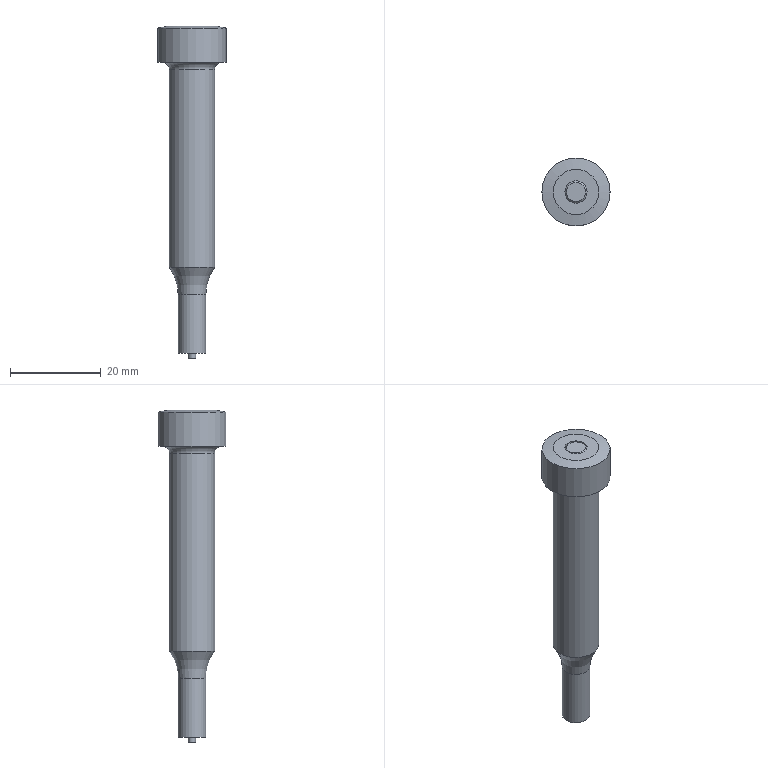Part | NX | features APJAS10-90-P6.08_2 2 | 1 solid | 20 faces | box 15 x 15 x 73 mm | volume 5513 mm3 | cylinder 8 | plane 7 | torus 2 | cone 2 | spline 1 | commonest cylinder face diameters 1.6 x1 1.8 x1 4.2 x1 4.4 x1 4.9 x1 6.08 x1
STEP:
#1=CARTESIAN_POINT('',(660.878,-22.569,60.5));
#2=VERTEX_POINT('',#1);
#3=CARTESIAN_POINT('',(665.878,-22.569,60.5));
#4=DIRECTION('',(0.,0.,1.));
#5=DIRECTION('',(1.,0.,0.));
#6=AXIS2_PLACEMENT_3D('',#3,#4,#5);
#7=CIRCLE('',#6,5.);
#8=EDGE_CURVE('',#2,#2,#7,.T.);
#9=ORIENTED_EDGE('',*,*,#8,.F.);
#10=EDGE_LOOP('',(#9));
#11=FACE_BOUND('',#10,.T.);
#12=CARTESIAN_POINT('',(670.878,-22.569,16.946));
#13=VERTEX_POINT('',#12);
#14=CARTESIAN_POINT('',(665.878,-22.569,16.946));
#15=DIRECTION('',(0.,0.,1.));
#16=DIRECTION('',(-1.,0.,0.));
#17=AXIS2_PLACEMENT_3D('',#14,#15,#16);
#18=CIRCLE('',#17,5.);
#19=EDGE_CURVE('',#13,#13,#18,.T.);
#20=ORIENTED_EDGE('',*,*,#19,.T.);
#21=EDGE_LOOP('',(#20));
#22=FACE_BOUND('',#21,.T.);
#23=CARTESIAN_POINT('',(665.878,-22.569,45.5));
#24=DIRECTION('',(0.,0.,-1.));
#25=DIRECTION('',(1.,0.,0.));
#26=AXIS2_PLACEMENT_3D('',#23,#24,#25);
#27=CYLINDRICAL_SURFACE('',#26,5.);
#28=ADVANCED_FACE('',(#11,#22),#27,.T.);
#29=CARTESIAN_POINT('',(664.978,-22.569,26.));
#30=VERTEX_POINT('',#29);
#31=CARTESIAN_POINT('',(665.878,-22.569,26.));
#32=DIRECTION('',(0.,0.,1.));
#33=DIRECTION('',(-1.,0.,0.));
#34=AXIS2_PLACEMENT_3D('',#31,#32,#33);
#35=CIRCLE('',#34,0.9);
#36=EDGE_CURVE('',#30,#30,#35,.T.);
#37=ORIENTED_EDGE('',*,*,#36,.T.);
#38=EDGE_LOOP('',(#37));
#39=FACE_BOUND('',#38,.T.);
#40=CARTESIAN_POINT('',(664.978,-22.569,-2.));
#41=VERTEX_POINT('',#40);
#42=CARTESIAN_POINT('',(665.878,-22.569,-2.));
#43=DIRECTION('',(0.,0.,1.));
#44=DIRECTION('',(-1.,0.,0.));
#45=AXIS2_PLACEMENT_3D('',#42,#43,#44);
#46=CIRCLE('',#45,0.9);
#47=EDGE_CURVE('',#41,#41,#46,.T.);
#48=ORIENTED_EDGE('',*,*,#47,.F.);
#49=EDGE_LOOP('',(#48));
#50=FACE_BOUND('',#49,.T.);
#51=CARTESIAN_POINT('',(665.878,-22.569,12.));
#52=DIRECTION('',(0.,0.,-1.));
#53=DIRECTION('',(1.,0.,0.));
#54=AXIS2_PLACEMENT_3D('',#51,#52,#53);
#55=CYLINDRICAL_SURFACE('',#54,0.9);
#56=ADVANCED_FACE('',(#39,#50),#55,.F.);
#57=CARTESIAN_POINT('',(668.328,-22.569,69.632));
#58=VERTEX_POINT('',#57);
#59=CARTESIAN_POINT('',(665.878,-22.569,69.632));
#60=DIRECTION('',(0.,0.,1.));
#61=DIRECTION('',(1.,0.,0.));
#62=AXIS2_PLACEMENT_3D('',#59,#60,#61);
#63=CIRCLE('',#62,2.45);
#64=EDGE_CURVE('',#58,#58,#63,.T.);
#65=ORIENTED_EDGE('',*,*,#64,.F.);
#66=EDGE_LOOP('',(#65));
#67=FACE_BOUND('',#66,.T.);
#68=CARTESIAN_POINT('',(663.428,-22.569,70.));
#69=VERTEX_POINT('',#68);
#70=CARTESIAN_POINT('',(665.878,-22.569,70.));
#71=DIRECTION('',(0.,0.,-1.));
#72=DIRECTION('',(-1.,0.,0.));
#73=AXIS2_PLACEMENT_3D('',#70,#71,#72);
#74=CIRCLE('',#73,2.45);
#75=EDGE_CURVE('',#69,#69,#74,.T.);
#76=ORIENTED_EDGE('',*,*,#75,.F.);
#77=EDGE_LOOP('',(#76));
#78=FACE_BOUND('',#77,.T.);
#79=CARTESIAN_POINT('',(665.878,-22.569,68.775));
#80=DIRECTION('',(0.,0.,-1.));
#81=DIRECTION('',(1.,0.,0.));
#82=AXIS2_PLACEMENT_3D('',#79,#80,#81);
#83=CYLINDRICAL_SURFACE('',#82,2.45);
#84=ADVANCED_FACE('',(#67,#78),#83,.F.);
#85=ORIENTED_EDGE('',*,*,#8,.T.);
#86=EDGE_LOOP('',(#85));
#87=FACE_BOUND('',#86,.T.);
#88=CARTESIAN_POINT('',(659.378,-22.569,62.));
#89=VERTEX_POINT('',#88);
#90=CARTESIAN_POINT('',(665.878,-22.569,62.));
#91=DIRECTION('',(0.,0.,-1.));
#92=DIRECTION('',(1.,0.,0.));
#93=AXIS2_PLACEMENT_3D('',#90,#91,#92);
#94=CIRCLE('',#93,6.5);
#95=EDGE_CURVE('',#89,#89,#94,.T.);
#96=ORIENTED_EDGE('',*,*,#95,.T.);
#97=EDGE_LOOP('',(#96));
#98=FACE_BOUND('',#97,.T.);
#99=CARTESIAN_POINT('',(665.878,-22.569,60.5));
#100=DIRECTION('',(0.,0.,1.));
#101=DIRECTION('',(-1.,0.,0.));
#102=AXIS2_PLACEMENT_3D('',#99,#100,#101);
#103=TOROIDAL_SURFACE('',#102,6.5,1.5);
#104=ADVANCED_FACE('',(#87,#98),#103,.F.);
#105=CARTESIAN_POINT('',(658.378,-22.569,62.));
#106=VERTEX_POINT('',#105);
#107=CARTESIAN_POINT('',(665.878,-22.569,62.));
#108=DIRECTION('',(0.,0.,-1.));
#109=DIRECTION('',(-1.,0.,0.));
#110=AXIS2_PLACEMENT_3D('',#107,#108,#109);
#111=CIRCLE('',#110,7.5);
#112=EDGE_CURVE('',#106,#106,#111,.T.);
#113=ORIENTED_EDGE('',*,*,#112,.T.);
#114=EDGE_LOOP('',(#113));
#115=FACE_BOUND('',#114,.T.);
#116=ORIENTED_EDGE('',*,*,#95,.F.);
#117=EDGE_LOOP('',(#116));
#118=FACE_BOUND('',#117,.T.);
#119=CARTESIAN_POINT('',(665.878,-22.569,62.));
#120=DIRECTION('',(0.,0.,-1.));
#121=DIRECTION('',(1.,0.,0.));
#122=AXIS2_PLACEMENT_3D('',#119,#120,#121);
#123=PLANE('',#122);
#124=ADVANCED_FACE('',(#115,#118),#123,.T.);
#125=CARTESIAN_POINT('',(662.838,-22.569,11.));
#126=VERTEX_POINT('',#125);
#127=CARTESIAN_POINT('',(665.878,-22.569,11.));
#128=DIRECTION('',(0.,0.,1.));
#129=DIRECTION('',(-1.,0.,0.));
#130=AXIS2_PLACEMENT_3D('',#127,#128,#129);
#131=CIRCLE('',#130,3.04);
#132=EDGE_CURVE('',#126,#126,#131,.T.);
#133=ORIENTED_EDGE('',*,*,#132,.T.);
#134=EDGE_LOOP('',(#133));
#135=FACE_BOUND('',#134,.T.);
#136=ORIENTED_EDGE('',*,*,#19,.F.);
#137=EDGE_LOOP('',(#136));
#138=FACE_BOUND('',#137,.T.);
#139=CARTESIAN_POINT('',(665.878,-22.569,11.));
#140=DIRECTION('',(0.,0.,-1.));
#141=DIRECTION('',(1.,0.,0.));
#142=AXIS2_PLACEMENT_3D('',#139,#140,#141);
#143=TOROIDAL_SURFACE('',#142,13.04,10.);
#144=ADVANCED_FACE('',(#135,#138),#143,.F.);
#145=CARTESIAN_POINT('',(658.378,-22.569,69.559));
#146=VERTEX_POINT('',#145);
#147=CARTESIAN_POINT('',(665.878,-22.569,69.559));
#148=DIRECTION('',(0.,0.,1.));
#149=DIRECTION('',(1.,0.,0.));
#150=AXIS2_PLACEMENT_3D('',#147,#148,#149);
#151=CIRCLE('',#150,7.5);
#152=EDGE_CURVE('',#146,#146,#151,.T.);
#153=ORIENTED_EDGE('',*,*,#152,.T.);
#154=EDGE_LOOP('',(#153));
#155=FACE_BOUND('',#154,.T.);
#156=CARTESIAN_POINT('',(660.878,-22.569,70.));
#157=VERTEX_POINT('',#156);
#158=CARTESIAN_POINT('',(665.878,-22.569,70.));
#159=DIRECTION('',(0.,0.,-1.));
#160=DIRECTION('',(1.,0.,0.));
#161=AXIS2_PLACEMENT_3D('',#158,#159,#160);
#162=CIRCLE('',#161,5.);
#163=EDGE_CURVE('',#157,#157,#162,.T.);
#164=ORIENTED_EDGE('',*,*,#163,.T.);
#165=EDGE_LOOP('',(#164));
#166=FACE_BOUND('',#165,.T.);
#167=CARTESIAN_POINT('',(665.878,-22.569,70.));
#168=DIRECTION('',(0.,0.,-1.));
#169=DIRECTION('',(-1.,0.,0.));
#170=AXIS2_PLACEMENT_3D('',#167,#168,#169);
#171=CONICAL_SURFACE('',#170,5.,1.396);
#172=ADVANCED_FACE('',(#155,#166),#171,.T.);
#173=ORIENTED_EDGE('',*,*,#112,.F.);
#174=EDGE_LOOP('',(#173));
#175=FACE_BOUND('',#174,.T.);
#176=ORIENTED_EDGE('',*,*,#152,.F.);
#177=EDGE_LOOP('',(#176));
#178=FACE_BOUND('',#177,.T.);
#179=CARTESIAN_POINT('',(665.878,-22.569,66.));
#180=DIRECTION('',(0.,0.,-1.));
#181=DIRECTION('',(1.,0.,0.));
#182=AXIS2_PLACEMENT_3D('',#179,#180,#181);
#183=CYLINDRICAL_SURFACE('',#182,7.5);
#184=ADVANCED_FACE('',(#175,#178),#183,.T.);
#185=ORIENTED_EDGE('',*,*,#75,.T.);
#186=EDGE_LOOP('',(#185));
#187=FACE_BOUND('',#186,.T.);
#188=ORIENTED_EDGE('',*,*,#163,.F.);
#189=EDGE_LOOP('',(#188));
#190=FACE_BOUND('',#189,.T.);
#191=CARTESIAN_POINT('',(665.878,-22.569,70.));
#192=DIRECTION('',(0.,0.,1.));
#193=DIRECTION('',(-1.,0.,0.));
#194=AXIS2_PLACEMENT_3D('',#191,#192,#193);
#195=PLANE('',#194);
#196=ADVANCED_FACE('',(#187,#190),#195,.T.);
#197=ORIENTED_EDGE('',*,*,#132,.F.);
#198=EDGE_LOOP('',(#197));
#199=FACE_BOUND('',#198,.T.);
#200=CARTESIAN_POINT('',(662.838,-22.569,-2.));
#201=VERTEX_POINT('',#200);
#202=CARTESIAN_POINT('',(665.878,-22.569,-2.));
#203=DIRECTION('',(0.,0.,-1.));
#204=DIRECTION('',(-1.,0.,0.));
#205=AXIS2_PLACEMENT_3D('',#202,#203,#204);
#206=CIRCLE('',#205,3.04);
#207=EDGE_CURVE('',#201,#201,#206,.T.);
#208=ORIENTED_EDGE('',*,*,#207,.F.);
#209=EDGE_LOOP('',(#208));
#210=FACE_BOUND('',#209,.T.);
#211=CARTESIAN_POINT('',(665.878,-22.569,4.5));
#212=DIRECTION('',(0.,0.,-1.));
#213=DIRECTION('',(1.,0.,0.));
#214=AXIS2_PLACEMENT_3D('',#211,#212,#213);
#215=CYLINDRICAL_SURFACE('',#214,3.04);
#216=ADVANCED_FACE('',(#199,#210),#215,.T.);
#217=ORIENTED_EDGE('',*,*,#47,.T.);
#218=EDGE_LOOP('',(#217));
#219=FACE_BOUND('',#218,.T.);
#220=ORIENTED_EDGE('',*,*,#207,.T.);
#221=EDGE_LOOP('',(#220));
#222=FACE_BOUND('',#221,.T.);
#223=CARTESIAN_POINT('',(665.878,-22.569,-2.));
#224=DIRECTION('',(0.,0.,-1.));
#225=DIRECTION('',(1.,0.,0.));
#226=AXIS2_PLACEMENT_3D('',#223,#224,#225);
#227=PLANE('',#226);
#228=ADVANCED_FACE('',(#219,#222),#227,.T.);
#229=CARTESIAN_POINT('',(667.96,-22.569,70.));
#230=VERTEX_POINT('',#229);
#231=CARTESIAN_POINT('',(665.878,-22.569,70.));
#232=DIRECTION('',(0.,0.,-1.));
#233=DIRECTION('',(1.,0.,0.));
#234=AXIS2_PLACEMENT_3D('',#231,#232,#233);
#235=CIRCLE('',#234,2.083);
#236=EDGE_CURVE('',#230,#230,#235,.T.);
#237=ORIENTED_EDGE('',*,*,#236,.F.);
#238=EDGE_LOOP('',(#237));
#239=FACE_BOUND('',#238,.T.);
#240=CARTESIAN_POINT('',(665.878,-22.569,70.));
#241=DIRECTION('',(0.,0.,1.));
#242=DIRECTION('',(-1.,0.,0.));
#243=AXIS2_PLACEMENT_3D('',#240,#241,#242);
#244=PLANE('',#243);
#245=ADVANCED_FACE('',(#239),#244,.T.);
#246=ORIENTED_EDGE('',*,*,#64,.T.);
#247=EDGE_LOOP('',(#246));
#248=FACE_BOUND('',#247,.T.);
#249=ORIENTED_EDGE('',*,*,#236,.T.);
#250=EDGE_LOOP('',(#249));
#251=FACE_BOUND('',#250,.T.);
#252=CARTESIAN_POINT('',(665.878,-22.569,70.));
#253=DIRECTION('',(0.,0.,-1.));
#254=DIRECTION('',(-1.,0.,0.));
#255=AXIS2_PLACEMENT_3D('',#252,#253,#254);
#256=CONICAL_SURFACE('',#255,2.083,0.7854);
#257=ADVANCED_FACE('',(#248,#251),#256,.T.);
#258=CARTESIAN_POINT('',(665.078,-22.569,26.));
#259=VERTEX_POINT('',#258);
#260=CARTESIAN_POINT('',(665.878,-22.569,26.));
#261=DIRECTION('',(0.,0.,-1.));
#262=DIRECTION('',(-1.,0.,0.));
#263=AXIS2_PLACEMENT_3D('',#260,#261,#262);
#264=CIRCLE('',#263,0.8);
#265=EDGE_CURVE('',#259,#259,#264,.F.);
#266=ORIENTED_EDGE('',*,*,#265,.T.);
#267=EDGE_LOOP('',(#266));
#268=FACE_BOUND('',#267,.T.);
#269=ORIENTED_EDGE('',*,*,#36,.F.);
#270=EDGE_LOOP('',(#269));
#271=FACE_BOUND('',#270,.T.);
#272=CARTESIAN_POINT('',(665.878,-22.569,26.));
#273=DIRECTION('',(0.,0.,-1.));
#274=DIRECTION('',(1.,0.,0.));
#275=AXIS2_PLACEMENT_3D('',#272,#273,#274);
#276=PLANE('',#275);
#277=ADVANCED_FACE('',(#268,#271),#276,.T.);
#278=ORIENTED_EDGE('',*,*,#265,.F.);
#279=EDGE_LOOP('',(#278));
#280=FACE_BOUND('',#279,.T.);
#281=CARTESIAN_POINT('',(665.078,-22.569,-3.));
#282=VERTEX_POINT('',#281);
#283=CARTESIAN_POINT('',(665.878,-22.569,-3.));
#284=DIRECTION('',(0.,0.,-1.));
#285=DIRECTION('',(-1.,0.,0.));
#286=AXIS2_PLACEMENT_3D('',#283,#284,#285);
#287=CIRCLE('',#286,0.8);
#288=EDGE_CURVE('',#282,#282,#287,.T.);
#289=ORIENTED_EDGE('',*,*,#288,.F.);
#290=EDGE_LOOP('',(#289));
#291=FACE_BOUND('',#290,.T.);
#292=CARTESIAN_POINT('',(665.878,-22.569,11.5));
#293=DIRECTION('',(0.,0.,-1.));
#294=DIRECTION('',(1.,0.,0.));
#295=AXIS2_PLACEMENT_3D('',#292,#293,#294);
#296=CYLINDRICAL_SURFACE('',#295,0.8);
#297=ADVANCED_FACE('',(#280,#291),#296,.T.);
#298=ORIENTED_EDGE('',*,*,#288,.T.);
#299=EDGE_LOOP('',(#298));
#300=FACE_BOUND('',#299,.T.);
#301=CARTESIAN_POINT('',(665.878,-22.569,-3.));
#302=DIRECTION('',(0.,0.,-1.));
#303=DIRECTION('',(1.,0.,0.));
#304=AXIS2_PLACEMENT_3D('',#301,#302,#303);
#305=PLANE('',#304);
#306=ADVANCED_FACE('',(#300),#305,.T.);
#307=CLOSED_SHELL('',(#28,#56,#84,#104,#124,#144,#172,#184,#196,#216,#228,#245,#257,#277,#297,#306));
#308=CARTESIAN_POINT('',(668.078,-22.567,65.1));
#309=VERTEX_POINT('',#308);
#310=CARTESIAN_POINT('',(667.601,-24.293,65.1));
#311=CARTESIAN_POINT('',(668.317,-22.567,65.1));
#312=CARTESIAN_POINT('',(667.598,-20.842,65.1));
#313=CARTESIAN_POINT('',(665.876,-20.131,65.1));
#314=CARTESIAN_POINT('',(664.151,-20.848,65.1));
#315=CARTESIAN_POINT('',(663.44,-22.571,65.1));
#316=CARTESIAN_POINT('',(664.154,-24.293,65.1));
#317=CARTESIAN_POINT('',(665.88,-25.007,65.1));
#318=CARTESIAN_POINT('',(667.601,-24.293,65.1));
#319=CARTESIAN_POINT('',(668.317,-22.567,65.1));
#320=CARTESIAN_POINT('',(667.598,-20.842,65.1));
#321=B_SPLINE_CURVE_WITH_KNOTS('',3,(#310,#311,#312,#313,#314,#315,#316,#317,#318,#319,#320),.UNSPECIFIED.,.T.,.F.,(1,1,1,1,1,1,1,1,1,1,1,1,1,1,1),(-0.00518,-0.003453,-0.001727,0.,0.001727,0.003453,0.00518,0.006907,0.008633,0.01036,0.01209,0.01381,0.01554,0.01727,0.01899),.UNSPECIFIED.);
#322=EDGE_CURVE('',#309,#309,#321,.T.);
#323=ORIENTED_EDGE('',*,*,#322,.T.);
#324=EDGE_LOOP('',(#323));
#325=FACE_BOUND('',#324,.T.);
#326=CARTESIAN_POINT('',(663.678,-22.569,26.));
#327=VERTEX_POINT('',#326);
#328=CARTESIAN_POINT('',(665.878,-22.569,26.));
#329=DIRECTION('',(0.,0.,-1.));
#330=DIRECTION('',(-1.,0.,0.));
#331=AXIS2_PLACEMENT_3D('',#328,#329,#330);
#332=CIRCLE('',#331,2.2);
#333=EDGE_CURVE('',#327,#327,#332,.T.);
#334=ORIENTED_EDGE('',*,*,#333,.T.);
#335=EDGE_LOOP('',(#334));
#336=FACE_BOUND('',#335,.T.);
#337=CARTESIAN_POINT('',(665.878,-22.569,55.775));
#338=DIRECTION('',(0.,0.,-1.));
#339=DIRECTION('',(1.,0.,0.));
#340=AXIS2_PLACEMENT_3D('',#337,#338,#339);
#341=CYLINDRICAL_SURFACE('',#340,2.2);
#342=ADVANCED_FACE('',(#325,#336),#341,.F.);
#343=CARTESIAN_POINT('',(663.778,-22.569,26.));
#344=VERTEX_POINT('',#343);
#345=CARTESIAN_POINT('',(665.878,-22.569,26.));
#346=DIRECTION('',(0.,0.,-1.));
#347=DIRECTION('',(-1.,0.,0.));
#348=AXIS2_PLACEMENT_3D('',#345,#346,#347);
#349=CIRCLE('',#348,2.1);
#350=EDGE_CURVE('',#344,#344,#349,.T.);
#351=ORIENTED_EDGE('',*,*,#350,.T.);
#352=EDGE_LOOP('',(#351));
#353=FACE_BOUND('',#352,.T.);
#354=ORIENTED_EDGE('',*,*,#333,.F.);
#355=EDGE_LOOP('',(#354));
#356=FACE_BOUND('',#355,.T.);
#357=CARTESIAN_POINT('',(665.878,-22.569,26.));
#358=DIRECTION('',(0.,0.,-1.));
#359=DIRECTION('',(1.,0.,0.));
#360=AXIS2_PLACEMENT_3D('',#357,#358,#359);
#361=PLANE('',#360);
#362=ADVANCED_FACE('',(#353,#356),#361,.F.);
#363=ORIENTED_EDGE('',*,*,#322,.F.);
#364=CARTESIAN_POINT('',(667.978,-22.567,64.961));
#365=VERTEX_POINT('',#364);
#366=CARTESIAN_POINT('',(668.328,-22.567,65.448));
#367=DIRECTION('',(-0.5832,-0.0004724,-0.8123));
#368=VECTOR('',#367,1000.);
#369=LINE('',#366,#368);
#370=EDGE_CURVE('',#309,#365,#369,.T.);
#371=ORIENTED_EDGE('',*,*,#370,.T.);
#372=CARTESIAN_POINT('',(667.978,-22.569,64.961));
#373=VERTEX_POINT('',#372);
#374=CARTESIAN_POINT('',(667.978,-22.567,64.961));
#375=CARTESIAN_POINT('',(667.977,-22.013,64.961));
#376=CARTESIAN_POINT('',(667.52,-20.924,64.961));
#377=CARTESIAN_POINT('',(665.877,-20.241,64.961));
#378=CARTESIAN_POINT('',(664.23,-20.925,64.961));
#379=CARTESIAN_POINT('',(663.551,-22.57,64.961));
#380=CARTESIAN_POINT('',(664.231,-24.213,64.961));
#381=CARTESIAN_POINT('',(665.878,-24.897,64.961));
#382=CARTESIAN_POINT('',(667.522,-24.213,64.961));
#383=CARTESIAN_POINT('',(667.978,-23.124,64.961));
#384=CARTESIAN_POINT('',(667.978,-22.569,64.961));
#385=B_SPLINE_CURVE_WITH_KNOTS('',3,(#374,#375,#376,#377,#378,#379,#380,#381,#382,#383,#384),.UNSPECIFIED.,.F.,.F.,(4,1,1,1,1,1,1,1,4),(0.,0.001646,0.003293,0.004939,0.006585,0.008232,0.009878,0.01152,0.01317),.UNSPECIFIED.);
#386=EDGE_CURVE('',#365,#373,#385,.T.);
#387=ORIENTED_EDGE('',*,*,#386,.T.);
#388=CARTESIAN_POINT('',(667.978,-22.569,64.961));
#389=CARTESIAN_POINT('',(667.978,-22.569,64.961));
#390=CARTESIAN_POINT('',(667.978,-22.568,64.961));
#391=CARTESIAN_POINT('',(667.978,-22.567,64.961));
#392=B_SPLINE_CURVE_WITH_KNOTS('',3,(#388,#389,#390,#391),.UNSPECIFIED.,.F.,.F.,(4,4),(0.004154,0.004156),.UNSPECIFIED.);
#393=EDGE_CURVE('',#373,#365,#392,.T.);
#394=ORIENTED_EDGE('',*,*,#393,.T.);
#395=ORIENTED_EDGE('',*,*,#370,.F.);
#396=EDGE_LOOP('',(#363,#371,#387,#394,#395));
#397=FACE_BOUND('',#396,.T.);
#398=CARTESIAN_POINT('',(667.977,-22.84,64.96));
#399=CARTESIAN_POINT('',(667.977,-22.84,64.96));
#400=CARTESIAN_POINT('',(667.977,-22.84,64.96));
#401=CARTESIAN_POINT('',(667.978,-22.84,64.961));
#402=CARTESIAN_POINT('',(668.01,-22.844,65.006));
#403=CARTESIAN_POINT('',(668.043,-22.848,65.051));
#404=CARTESIAN_POINT('',(668.075,-22.853,65.097));
#405=CARTESIAN_POINT('',(668.076,-22.853,65.098));
#406=CARTESIAN_POINT('',(668.077,-22.853,65.099));
#407=CARTESIAN_POINT('',(668.078,-22.853,65.1));
#408=CARTESIAN_POINT('',(668.078,-22.853,65.101));
#409=CARTESIAN_POINT('',(668.078,-22.853,65.101));
#410=CARTESIAN_POINT('',(668.079,-22.853,65.102));
#411=CARTESIAN_POINT('',(667.977,-22.415,64.96));
#412=CARTESIAN_POINT('',(667.977,-22.415,64.96));
#413=CARTESIAN_POINT('',(667.977,-22.415,64.96));
#414=CARTESIAN_POINT('',(667.978,-22.415,64.961));
#415=CARTESIAN_POINT('',(668.01,-22.412,65.006));
#416=CARTESIAN_POINT('',(668.043,-22.41,65.051));
#417=CARTESIAN_POINT('',(668.075,-22.408,65.097));
#418=CARTESIAN_POINT('',(668.076,-22.408,65.098));
#419=CARTESIAN_POINT('',(668.077,-22.408,65.099));
#420=CARTESIAN_POINT('',(668.078,-22.407,65.1));
#421=CARTESIAN_POINT('',(668.078,-22.407,65.101));
#422=CARTESIAN_POINT('',(668.078,-22.407,65.101));
#423=CARTESIAN_POINT('',(668.079,-22.407,65.102));
#424=CARTESIAN_POINT('',(667.96,-22.26,64.96));
#425=CARTESIAN_POINT('',(667.96,-22.26,64.96));
#426=CARTESIAN_POINT('',(667.96,-22.26,64.96));
#427=CARTESIAN_POINT('',(667.96,-22.26,64.961));
#428=CARTESIAN_POINT('',(667.993,-22.255,65.006));
#429=CARTESIAN_POINT('',(668.025,-22.25,65.051));
#430=CARTESIAN_POINT('',(668.057,-22.245,65.097));
#431=CARTESIAN_POINT('',(668.058,-22.245,65.098));
#432=CARTESIAN_POINT('',(668.059,-22.245,65.099));
#433=CARTESIAN_POINT('',(668.06,-22.245,65.1));
#434=CARTESIAN_POINT('',(668.06,-22.245,65.101));
#435=CARTESIAN_POINT('',(668.06,-22.245,65.101));
#436=CARTESIAN_POINT('',(668.061,-22.245,65.102));
#437=CARTESIAN_POINT('',(667.892,-21.959,64.96));
#438=CARTESIAN_POINT('',(667.892,-21.958,64.96));
#439=CARTESIAN_POINT('',(667.893,-21.958,64.96));
#440=CARTESIAN_POINT('',(667.893,-21.958,64.961));
#441=CARTESIAN_POINT('',(667.924,-21.949,65.006));
#442=CARTESIAN_POINT('',(667.955,-21.939,65.051));
#443=CARTESIAN_POINT('',(667.986,-21.93,65.097));
#444=CARTESIAN_POINT('',(667.987,-21.93,65.098));
#445=CARTESIAN_POINT('',(667.988,-21.929,65.099));
#446=CARTESIAN_POINT('',(667.989,-21.929,65.1));
#447=CARTESIAN_POINT('',(667.989,-21.929,65.101));
#448=CARTESIAN_POINT('',(667.99,-21.929,65.101));
#449=CARTESIAN_POINT('',(667.99,-21.929,65.102));
#450=CARTESIAN_POINT('',(667.841,-21.811,64.96));
#451=CARTESIAN_POINT('',(667.841,-21.811,64.96));
#452=CARTESIAN_POINT('',(667.842,-21.811,64.96));
#453=CARTESIAN_POINT('',(667.842,-21.811,64.961));
#454=CARTESIAN_POINT('',(667.872,-21.799,65.006));
#455=CARTESIAN_POINT('',(667.903,-21.787,65.051));
#456=CARTESIAN_POINT('',(667.933,-21.775,65.097));
#457=CARTESIAN_POINT('',(667.934,-21.775,65.098));
#458=CARTESIAN_POINT('',(667.935,-21.775,65.099));
#459=CARTESIAN_POINT('',(667.936,-21.774,65.1));
#460=CARTESIAN_POINT('',(667.936,-21.774,65.101));
#461=CARTESIAN_POINT('',(667.936,-21.774,65.101));
#462=CARTESIAN_POINT('',(667.937,-21.774,65.102));
#463=CARTESIAN_POINT('',(667.659,-21.427,64.96));
#464=CARTESIAN_POINT('',(667.66,-21.427,64.96));
#465=CARTESIAN_POINT('',(667.66,-21.426,64.96));
#466=CARTESIAN_POINT('',(667.66,-21.426,64.961));
#467=CARTESIAN_POINT('',(667.688,-21.409,65.006));
#468=CARTESIAN_POINT('',(667.715,-21.391,65.051));
#469=CARTESIAN_POINT('',(667.743,-21.373,65.097));
#470=CARTESIAN_POINT('',(667.744,-21.373,65.098));
#471=CARTESIAN_POINT('',(667.744,-21.372,65.099));
#472=CARTESIAN_POINT('',(667.745,-21.372,65.1));
#473=CARTESIAN_POINT('',(667.745,-21.372,65.101));
#474=CARTESIAN_POINT('',(667.746,-21.371,65.101));
#475=CARTESIAN_POINT('',(667.746,-21.371,65.102));
#476=CARTESIAN_POINT('',(667.492,-21.201,64.96));
#477=CARTESIAN_POINT('',(667.493,-21.201,64.96));
#478=CARTESIAN_POINT('',(667.493,-21.2,64.96));
#479=CARTESIAN_POINT('',(667.493,-21.2,64.961));
#480=CARTESIAN_POINT('',(667.518,-21.179,65.006));
#481=CARTESIAN_POINT('',(667.543,-21.158,65.051));
#482=CARTESIAN_POINT('',(667.568,-21.137,65.097));
#483=CARTESIAN_POINT('',(667.569,-21.136,65.098));
#484=CARTESIAN_POINT('',(667.569,-21.136,65.099));
#485=CARTESIAN_POINT('',(667.57,-21.135,65.1));
#486=CARTESIAN_POINT('',(667.57,-21.135,65.101));
#487=CARTESIAN_POINT('',(667.571,-21.134,65.101));
#488=CARTESIAN_POINT('',(667.571,-21.134,65.102));
#489=CARTESIAN_POINT('',(667.092,-20.836,64.96));
#490=CARTESIAN_POINT('',(667.092,-20.836,64.96));
#491=CARTESIAN_POINT('',(667.093,-20.835,64.96));
#492=CARTESIAN_POINT('',(667.093,-20.835,64.961));
#493=CARTESIAN_POINT('',(667.112,-20.808,65.006));
#494=CARTESIAN_POINT('',(667.13,-20.781,65.051));
#495=CARTESIAN_POINT('',(667.149,-20.755,65.097));
#496=CARTESIAN_POINT('',(667.15,-20.754,65.098));
#497=CARTESIAN_POINT('',(667.15,-20.753,65.099));
#498=CARTESIAN_POINT('',(667.151,-20.753,65.1));
#499=CARTESIAN_POINT('',(667.151,-20.752,65.101));
#500=CARTESIAN_POINT('',(667.151,-20.752,65.101));
#501=CARTESIAN_POINT('',(667.151,-20.752,65.102));
#502=CARTESIAN_POINT('',(666.852,-20.69,64.96));
#503=CARTESIAN_POINT('',(666.852,-20.69,64.96));
#504=CARTESIAN_POINT('',(666.852,-20.69,64.96));
#505=CARTESIAN_POINT('',(666.852,-20.689,64.961));
#506=CARTESIAN_POINT('',(666.867,-20.66,65.006));
#507=CARTESIAN_POINT('',(666.882,-20.631,65.051));
#508=CARTESIAN_POINT('',(666.898,-20.602,65.097));
#509=CARTESIAN_POINT('',(666.898,-20.601,65.098));
#510=CARTESIAN_POINT('',(666.898,-20.601,65.099));
#511=CARTESIAN_POINT('',(666.899,-20.6,65.1));
#512=CARTESIAN_POINT('',(666.899,-20.6,65.101));
#513=CARTESIAN_POINT('',(666.899,-20.599,65.101));
#514=CARTESIAN_POINT('',(666.899,-20.599,65.102));
#515=CARTESIAN_POINT('',(666.343,-20.504,64.96));
#516=CARTESIAN_POINT('',(666.343,-20.504,64.96));
#517=CARTESIAN_POINT('',(666.343,-20.504,64.96));
#518=CARTESIAN_POINT('',(666.343,-20.504,64.961));
#519=CARTESIAN_POINT('',(666.351,-20.472,65.006));
#520=CARTESIAN_POINT('',(666.358,-20.44,65.051));
#521=CARTESIAN_POINT('',(666.365,-20.408,65.097));
#522=CARTESIAN_POINT('',(666.365,-20.407,65.098));
#523=CARTESIAN_POINT('',(666.365,-20.406,65.099));
#524=CARTESIAN_POINT('',(666.366,-20.405,65.1));
#525=CARTESIAN_POINT('',(666.366,-20.405,65.101));
#526=CARTESIAN_POINT('',(666.366,-20.405,65.101));
#527=CARTESIAN_POINT('',(666.366,-20.404,65.102));
#528=CARTESIAN_POINT('',(666.066,-20.461,64.96));
#529=CARTESIAN_POINT('',(666.066,-20.461,64.96));
#530=CARTESIAN_POINT('',(666.066,-20.46,64.96));
#531=CARTESIAN_POINT('',(666.066,-20.46,64.961));
#532=CARTESIAN_POINT('',(666.069,-20.428,65.006));
#533=CARTESIAN_POINT('',(666.072,-20.395,65.051));
#534=CARTESIAN_POINT('',(666.074,-20.362,65.097));
#535=CARTESIAN_POINT('',(666.075,-20.361,65.098));
#536=CARTESIAN_POINT('',(666.075,-20.361,65.099));
#537=CARTESIAN_POINT('',(666.075,-20.36,65.1));
#538=CARTESIAN_POINT('',(666.075,-20.359,65.101));
#539=CARTESIAN_POINT('',(666.075,-20.359,65.101));
#540=CARTESIAN_POINT('',(666.075,-20.359,65.102));
#541=CARTESIAN_POINT('',(665.525,-20.482,64.96));
#542=CARTESIAN_POINT('',(665.524,-20.482,64.96));
#543=CARTESIAN_POINT('',(665.524,-20.482,64.96));
#544=CARTESIAN_POINT('',(665.524,-20.481,64.961));
#545=CARTESIAN_POINT('',(665.519,-20.449,65.006));
#546=CARTESIAN_POINT('',(665.513,-20.417,65.051));
#547=CARTESIAN_POINT('',(665.508,-20.385,65.097));
#548=CARTESIAN_POINT('',(665.508,-20.384,65.098));
#549=CARTESIAN_POINT('',(665.508,-20.383,65.099));
#550=CARTESIAN_POINT('',(665.508,-20.382,65.1));
#551=CARTESIAN_POINT('',(665.507,-20.382,65.101));
#552=CARTESIAN_POINT('',(665.507,-20.381,65.101));
#553=CARTESIAN_POINT('',(665.507,-20.381,65.102));
#554=CARTESIAN_POINT('',(665.251,-20.547,64.96));
#555=CARTESIAN_POINT('',(665.251,-20.547,64.96));
#556=CARTESIAN_POINT('',(665.251,-20.547,64.96));
#557=CARTESIAN_POINT('',(665.251,-20.547,64.961));
#558=CARTESIAN_POINT('',(665.241,-20.515,65.006));
#559=CARTESIAN_POINT('',(665.232,-20.484,65.051));
#560=CARTESIAN_POINT('',(665.222,-20.453,65.097));
#561=CARTESIAN_POINT('',(665.222,-20.452,65.098));
#562=CARTESIAN_POINT('',(665.221,-20.451,65.099));
#563=CARTESIAN_POINT('',(665.221,-20.45,65.1));
#564=CARTESIAN_POINT('',(665.221,-20.45,65.101));
#565=CARTESIAN_POINT('',(665.221,-20.45,65.101));
#566=CARTESIAN_POINT('',(665.221,-20.449,65.102));
#567=CARTESIAN_POINT('',(664.759,-20.773,64.96));
#568=CARTESIAN_POINT('',(664.759,-20.772,64.96));
#569=CARTESIAN_POINT('',(664.758,-20.772,64.96));
#570=CARTESIAN_POINT('',(664.758,-20.772,64.961));
#571=CARTESIAN_POINT('',(664.741,-20.744,65.006));
#572=CARTESIAN_POINT('',(664.724,-20.716,65.051));
#573=CARTESIAN_POINT('',(664.706,-20.688,65.097));
#574=CARTESIAN_POINT('',(664.706,-20.688,65.098));
#575=CARTESIAN_POINT('',(664.705,-20.687,65.099));
#576=CARTESIAN_POINT('',(664.705,-20.686,65.1));
#577=CARTESIAN_POINT('',(664.705,-20.686,65.101));
#578=CARTESIAN_POINT('',(664.704,-20.686,65.101));
#579=CARTESIAN_POINT('',(664.704,-20.685,65.102));
#580=CARTESIAN_POINT('',(664.531,-20.937,64.96));
#581=CARTESIAN_POINT('',(664.53,-20.936,64.96));
#582=CARTESIAN_POINT('',(664.53,-20.936,64.96));
#583=CARTESIAN_POINT('',(664.53,-20.936,64.961));
#584=CARTESIAN_POINT('',(664.509,-20.911,65.006));
#585=CARTESIAN_POINT('',(664.488,-20.885,65.051));
#586=CARTESIAN_POINT('',(664.467,-20.86,65.097));
#587=CARTESIAN_POINT('',(664.467,-20.86,65.098));
#588=CARTESIAN_POINT('',(664.466,-20.859,65.099));
#589=CARTESIAN_POINT('',(664.466,-20.858,65.1));
#590=CARTESIAN_POINT('',(664.466,-20.858,65.101));
#591=CARTESIAN_POINT('',(664.465,-20.858,65.101));
#592=CARTESIAN_POINT('',(664.465,-20.857,65.102));
#593=CARTESIAN_POINT('',(664.16,-21.332,64.96));
#594=CARTESIAN_POINT('',(664.16,-21.332,64.96));
#595=CARTESIAN_POINT('',(664.16,-21.332,64.96));
#596=CARTESIAN_POINT('',(664.16,-21.331,64.961));
#597=CARTESIAN_POINT('',(664.133,-21.312,65.006));
#598=CARTESIAN_POINT('',(664.107,-21.293,65.051));
#599=CARTESIAN_POINT('',(664.08,-21.274,65.097));
#600=CARTESIAN_POINT('',(664.079,-21.274,65.098));
#601=CARTESIAN_POINT('',(664.079,-21.273,65.099));
#602=CARTESIAN_POINT('',(664.078,-21.273,65.1));
#603=CARTESIAN_POINT('',(664.078,-21.272,65.101));
#604=CARTESIAN_POINT('',(664.077,-21.272,65.101));
#605=CARTESIAN_POINT('',(664.077,-21.272,65.102));
#606=CARTESIAN_POINT('',(664.012,-21.57,64.96));
#607=CARTESIAN_POINT('',(664.011,-21.57,64.96));
#608=CARTESIAN_POINT('',(664.011,-21.57,64.96));
#609=CARTESIAN_POINT('',(664.011,-21.57,64.961));
#610=CARTESIAN_POINT('',(663.982,-21.555,65.006));
#611=CARTESIAN_POINT('',(663.953,-21.539,65.051));
#612=CARTESIAN_POINT('',(663.924,-21.524,65.097));
#613=CARTESIAN_POINT('',(663.923,-21.523,65.098));
#614=CARTESIAN_POINT('',(663.923,-21.523,65.099));
#615=CARTESIAN_POINT('',(663.922,-21.522,65.1));
#616=CARTESIAN_POINT('',(663.922,-21.522,65.101));
#617=CARTESIAN_POINT('',(663.921,-21.522,65.101));
#618=CARTESIAN_POINT('',(663.921,-21.522,65.102));
#619=CARTESIAN_POINT('',(663.819,-22.077,64.96));
#620=CARTESIAN_POINT('',(663.819,-22.077,64.96));
#621=CARTESIAN_POINT('',(663.819,-22.076,64.96));
#622=CARTESIAN_POINT('',(663.818,-22.076,64.961));
#623=CARTESIAN_POINT('',(663.787,-22.069,65.006));
#624=CARTESIAN_POINT('',(663.755,-22.061,65.051));
#625=CARTESIAN_POINT('',(663.723,-22.054,65.097));
#626=CARTESIAN_POINT('',(663.722,-22.053,65.098));
#627=CARTESIAN_POINT('',(663.721,-22.053,65.099));
#628=CARTESIAN_POINT('',(663.72,-22.053,65.1));
#629=CARTESIAN_POINT('',(663.72,-22.053,65.101));
#630=CARTESIAN_POINT('',(663.72,-22.053,65.101));
#631=CARTESIAN_POINT('',(663.719,-22.053,65.102));
#632=CARTESIAN_POINT('',(663.772,-22.354,64.96));
#633=CARTESIAN_POINT('',(663.772,-22.354,64.96));
#634=CARTESIAN_POINT('',(663.772,-22.354,64.96));
#635=CARTESIAN_POINT('',(663.771,-22.354,64.961));
#636=CARTESIAN_POINT('',(663.739,-22.35,65.006));
#637=CARTESIAN_POINT('',(663.706,-22.347,65.051));
#638=CARTESIAN_POINT('',(663.674,-22.343,65.097));
#639=CARTESIAN_POINT('',(663.673,-22.343,65.098));
#640=CARTESIAN_POINT('',(663.672,-22.343,65.099));
#641=CARTESIAN_POINT('',(663.671,-22.343,65.1));
#642=CARTESIAN_POINT('',(663.671,-22.343,65.101));
#643=CARTESIAN_POINT('',(663.67,-22.343,65.101));
#644=CARTESIAN_POINT('',(663.67,-22.343,65.102));
#645=CARTESIAN_POINT('',(663.786,-22.895,64.96));
#646=CARTESIAN_POINT('',(663.786,-22.895,64.96));
#647=CARTESIAN_POINT('',(663.786,-22.895,64.96));
#648=CARTESIAN_POINT('',(663.786,-22.895,64.961));
#649=CARTESIAN_POINT('',(663.753,-22.9,65.006));
#650=CARTESIAN_POINT('',(663.721,-22.905,65.051));
#651=CARTESIAN_POINT('',(663.688,-22.91,65.097));
#652=CARTESIAN_POINT('',(663.688,-22.91,65.098));
#653=CARTESIAN_POINT('',(663.687,-22.91,65.099));
#654=CARTESIAN_POINT('',(663.686,-22.911,65.1));
#655=CARTESIAN_POINT('',(663.685,-22.911,65.101));
#656=CARTESIAN_POINT('',(663.685,-22.911,65.101));
#657=CARTESIAN_POINT('',(663.685,-22.911,65.102));
#658=CARTESIAN_POINT('',(663.848,-23.169,64.96));
#659=CARTESIAN_POINT('',(663.848,-23.169,64.96));
#660=CARTESIAN_POINT('',(663.847,-23.169,64.96));
#661=CARTESIAN_POINT('',(663.847,-23.169,64.961));
#662=CARTESIAN_POINT('',(663.816,-23.179,65.006));
#663=CARTESIAN_POINT('',(663.784,-23.188,65.051));
#664=CARTESIAN_POINT('',(663.753,-23.197,65.097));
#665=CARTESIAN_POINT('',(663.752,-23.197,65.098));
#666=CARTESIAN_POINT('',(663.751,-23.198,65.099));
#667=CARTESIAN_POINT('',(663.75,-23.198,65.1));
#668=CARTESIAN_POINT('',(663.75,-23.198,65.101));
#669=CARTESIAN_POINT('',(663.75,-23.198,65.101));
#670=CARTESIAN_POINT('',(663.749,-23.198,65.102));
#671=CARTESIAN_POINT('',(664.067,-23.665,64.96));
#672=CARTESIAN_POINT('',(664.066,-23.665,64.96));
#673=CARTESIAN_POINT('',(664.066,-23.665,64.96));
#674=CARTESIAN_POINT('',(664.066,-23.665,64.961));
#675=CARTESIAN_POINT('',(664.038,-23.682,65.006));
#676=CARTESIAN_POINT('',(664.01,-23.699,65.051));
#677=CARTESIAN_POINT('',(663.982,-23.716,65.097));
#678=CARTESIAN_POINT('',(663.981,-23.716,65.098));
#679=CARTESIAN_POINT('',(663.98,-23.717,65.099));
#680=CARTESIAN_POINT('',(663.98,-23.717,65.1));
#681=CARTESIAN_POINT('',(663.979,-23.717,65.101));
#682=CARTESIAN_POINT('',(663.979,-23.718,65.101));
#683=CARTESIAN_POINT('',(663.979,-23.718,65.102));
#684=CARTESIAN_POINT('',(664.228,-23.895,64.96));
#685=CARTESIAN_POINT('',(664.227,-23.895,64.96));
#686=CARTESIAN_POINT('',(664.227,-23.895,64.96));
#687=CARTESIAN_POINT('',(664.227,-23.895,64.961));
#688=CARTESIAN_POINT('',(664.201,-23.916,65.006));
#689=CARTESIAN_POINT('',(664.176,-23.936,65.051));
#690=CARTESIAN_POINT('',(664.15,-23.957,65.097));
#691=CARTESIAN_POINT('',(664.15,-23.957,65.098));
#692=CARTESIAN_POINT('',(664.149,-23.958,65.099));
#693=CARTESIAN_POINT('',(664.148,-23.958,65.1));
#694=CARTESIAN_POINT('',(664.148,-23.959,65.101));
#695=CARTESIAN_POINT('',(664.148,-23.959,65.101));
#696=CARTESIAN_POINT('',(664.147,-23.959,65.102));
#697=CARTESIAN_POINT('',(664.618,-24.27,64.96));
#698=CARTESIAN_POINT('',(664.618,-24.27,64.96));
#699=CARTESIAN_POINT('',(664.618,-24.271,64.96));
#700=CARTESIAN_POINT('',(664.618,-24.271,64.961));
#701=CARTESIAN_POINT('',(664.598,-24.297,65.006));
#702=CARTESIAN_POINT('',(664.579,-24.323,65.051));
#703=CARTESIAN_POINT('',(664.559,-24.35,65.097));
#704=CARTESIAN_POINT('',(664.559,-24.35,65.098));
#705=CARTESIAN_POINT('',(664.558,-24.351,65.099));
#706=CARTESIAN_POINT('',(664.558,-24.352,65.1));
#707=CARTESIAN_POINT('',(664.557,-24.352,65.101));
#708=CARTESIAN_POINT('',(664.557,-24.352,65.101));
#709=CARTESIAN_POINT('',(664.557,-24.353,65.102));
#710=CARTESIAN_POINT('',(664.854,-24.422,64.96));
#711=CARTESIAN_POINT('',(664.854,-24.422,64.96));
#712=CARTESIAN_POINT('',(664.854,-24.422,64.96));
#713=CARTESIAN_POINT('',(664.854,-24.423,64.961));
#714=CARTESIAN_POINT('',(664.838,-24.451,65.006));
#715=CARTESIAN_POINT('',(664.822,-24.48,65.051));
#716=CARTESIAN_POINT('',(664.807,-24.509,65.097));
#717=CARTESIAN_POINT('',(664.806,-24.51,65.098));
#718=CARTESIAN_POINT('',(664.806,-24.51,65.099));
#719=CARTESIAN_POINT('',(664.805,-24.511,65.1));
#720=CARTESIAN_POINT('',(664.805,-24.511,65.101));
#721=CARTESIAN_POINT('',(664.805,-24.512,65.101));
#722=CARTESIAN_POINT('',(664.805,-24.512,65.102));
#723=CARTESIAN_POINT('',(665.358,-24.621,64.96));
#724=CARTESIAN_POINT('',(665.358,-24.621,64.96));
#725=CARTESIAN_POINT('',(665.358,-24.622,64.96));
#726=CARTESIAN_POINT('',(665.358,-24.622,64.961));
#727=CARTESIAN_POINT('',(665.35,-24.654,65.006));
#728=CARTESIAN_POINT('',(665.342,-24.685,65.051));
#729=CARTESIAN_POINT('',(665.334,-24.717,65.097));
#730=CARTESIAN_POINT('',(665.334,-24.718,65.098));
#731=CARTESIAN_POINT('',(665.333,-24.719,65.099));
#732=CARTESIAN_POINT('',(665.333,-24.72,65.1));
#733=CARTESIAN_POINT('',(665.333,-24.72,65.101));
#734=CARTESIAN_POINT('',(665.333,-24.72,65.101));
#735=CARTESIAN_POINT('',(665.333,-24.721,65.102));
#736=CARTESIAN_POINT('',(665.634,-24.672,64.96));
#737=CARTESIAN_POINT('',(665.634,-24.672,64.96));
#738=CARTESIAN_POINT('',(665.634,-24.672,64.96));
#739=CARTESIAN_POINT('',(665.634,-24.673,64.961));
#740=CARTESIAN_POINT('',(665.631,-24.705,65.006));
#741=CARTESIAN_POINT('',(665.627,-24.738,65.051));
#742=CARTESIAN_POINT('',(665.623,-24.77,65.097));
#743=CARTESIAN_POINT('',(665.623,-24.771,65.098));
#744=CARTESIAN_POINT('',(665.623,-24.772,65.099));
#745=CARTESIAN_POINT('',(665.623,-24.773,65.1));
#746=CARTESIAN_POINT('',(665.623,-24.773,65.101));
#747=CARTESIAN_POINT('',(665.623,-24.774,65.101));
#748=CARTESIAN_POINT('',(665.623,-24.774,65.102));
#749=CARTESIAN_POINT('',(666.176,-24.665,64.96));
#750=CARTESIAN_POINT('',(666.176,-24.665,64.96));
#751=CARTESIAN_POINT('',(666.176,-24.665,64.96));
#752=CARTESIAN_POINT('',(666.176,-24.665,64.961));
#753=CARTESIAN_POINT('',(666.181,-24.698,65.006));
#754=CARTESIAN_POINT('',(666.185,-24.73,65.051));
#755=CARTESIAN_POINT('',(666.19,-24.763,65.097));
#756=CARTESIAN_POINT('',(666.19,-24.764,65.098));
#757=CARTESIAN_POINT('',(666.19,-24.764,65.099));
#758=CARTESIAN_POINT('',(666.19,-24.765,65.1));
#759=CARTESIAN_POINT('',(666.19,-24.766,65.101));
#760=CARTESIAN_POINT('',(666.19,-24.766,65.101));
#761=CARTESIAN_POINT('',(666.19,-24.766,65.102));
#762=CARTESIAN_POINT('',(666.451,-24.607,64.96));
#763=CARTESIAN_POINT('',(666.451,-24.607,64.96));
#764=CARTESIAN_POINT('',(666.451,-24.607,64.96));
#765=CARTESIAN_POINT('',(666.451,-24.607,64.961));
#766=CARTESIAN_POINT('',(666.46,-24.639,65.006));
#767=CARTESIAN_POINT('',(666.469,-24.671,65.051));
#768=CARTESIAN_POINT('',(666.478,-24.702,65.097));
#769=CARTESIAN_POINT('',(666.478,-24.703,65.098));
#770=CARTESIAN_POINT('',(666.478,-24.704,65.099));
#771=CARTESIAN_POINT('',(666.478,-24.705,65.1));
#772=CARTESIAN_POINT('',(666.479,-24.705,65.101));
#773=CARTESIAN_POINT('',(666.479,-24.705,65.101));
#774=CARTESIAN_POINT('',(666.479,-24.706,65.102));
#775=CARTESIAN_POINT('',(666.949,-24.395,64.96));
#776=CARTESIAN_POINT('',(666.949,-24.395,64.96));
#777=CARTESIAN_POINT('',(666.949,-24.395,64.96));
#778=CARTESIAN_POINT('',(666.95,-24.395,64.961));
#779=CARTESIAN_POINT('',(666.966,-24.423,65.006));
#780=CARTESIAN_POINT('',(666.983,-24.452,65.051));
#781=CARTESIAN_POINT('',(666.999,-24.48,65.097));
#782=CARTESIAN_POINT('',(667.,-24.481,65.098));
#783=CARTESIAN_POINT('',(667.,-24.481,65.099));
#784=CARTESIAN_POINT('',(667.001,-24.482,65.1));
#785=CARTESIAN_POINT('',(667.001,-24.483,65.101));
#786=CARTESIAN_POINT('',(667.001,-24.483,65.101));
#787=CARTESIAN_POINT('',(667.001,-24.483,65.102));
#788=CARTESIAN_POINT('',(667.182,-24.236,64.96));
#789=CARTESIAN_POINT('',(667.182,-24.237,64.96));
#790=CARTESIAN_POINT('',(667.182,-24.237,64.96));
#791=CARTESIAN_POINT('',(667.182,-24.237,64.961));
#792=CARTESIAN_POINT('',(667.202,-24.263,65.006));
#793=CARTESIAN_POINT('',(667.222,-24.289,65.051));
#794=CARTESIAN_POINT('',(667.243,-24.315,65.097));
#795=CARTESIAN_POINT('',(667.243,-24.315,65.098));
#796=CARTESIAN_POINT('',(667.244,-24.316,65.099));
#797=CARTESIAN_POINT('',(667.244,-24.317,65.1));
#798=CARTESIAN_POINT('',(667.244,-24.317,65.101));
#799=CARTESIAN_POINT('',(667.245,-24.317,65.101));
#800=CARTESIAN_POINT('',(667.245,-24.317,65.102));
#801=CARTESIAN_POINT('',(667.562,-23.851,64.96));
#802=CARTESIAN_POINT('',(667.562,-23.851,64.96));
#803=CARTESIAN_POINT('',(667.562,-23.851,64.96));
#804=CARTESIAN_POINT('',(667.563,-23.852,64.961));
#805=CARTESIAN_POINT('',(667.589,-23.871,65.006));
#806=CARTESIAN_POINT('',(667.615,-23.891,65.051));
#807=CARTESIAN_POINT('',(667.641,-23.911,65.097));
#808=CARTESIAN_POINT('',(667.641,-23.912,65.098));
#809=CARTESIAN_POINT('',(667.642,-23.912,65.099));
#810=CARTESIAN_POINT('',(667.643,-23.913,65.1));
#811=CARTESIAN_POINT('',(667.643,-23.913,65.101));
#812=CARTESIAN_POINT('',(667.643,-23.913,65.101));
#813=CARTESIAN_POINT('',(667.644,-23.913,65.102));
#814=CARTESIAN_POINT('',(667.717,-23.617,64.96));
#815=CARTESIAN_POINT('',(667.717,-23.617,64.96));
#816=CARTESIAN_POINT('',(667.717,-23.617,64.96));
#817=CARTESIAN_POINT('',(667.718,-23.617,64.961));
#818=CARTESIAN_POINT('',(667.746,-23.633,65.006));
#819=CARTESIAN_POINT('',(667.775,-23.649,65.051));
#820=CARTESIAN_POINT('',(667.803,-23.666,65.097));
#821=CARTESIAN_POINT('',(667.804,-23.666,65.098));
#822=CARTESIAN_POINT('',(667.805,-23.667,65.099));
#823=CARTESIAN_POINT('',(667.805,-23.667,65.1));
#824=CARTESIAN_POINT('',(667.806,-23.667,65.101));
#825=CARTESIAN_POINT('',(667.806,-23.667,65.101));
#826=CARTESIAN_POINT('',(667.806,-23.668,65.102));
#827=CARTESIAN_POINT('',(667.923,-23.116,64.96));
#828=CARTESIAN_POINT('',(667.923,-23.116,64.96));
#829=CARTESIAN_POINT('',(667.923,-23.116,64.96));
#830=CARTESIAN_POINT('',(667.923,-23.116,64.961));
#831=CARTESIAN_POINT('',(667.955,-23.124,65.006));
#832=CARTESIAN_POINT('',(667.987,-23.133,65.051));
#833=CARTESIAN_POINT('',(668.018,-23.141,65.097));
#834=CARTESIAN_POINT('',(668.019,-23.141,65.098));
#835=CARTESIAN_POINT('',(668.02,-23.142,65.099));
#836=CARTESIAN_POINT('',(668.021,-23.142,65.1));
#837=CARTESIAN_POINT('',(668.021,-23.142,65.101));
#838=CARTESIAN_POINT('',(668.021,-23.142,65.101));
#839=CARTESIAN_POINT('',(668.022,-23.142,65.102));
#840=CARTESIAN_POINT('',(667.977,-22.84,64.96));
#841=CARTESIAN_POINT('',(667.977,-22.84,64.96));
#842=CARTESIAN_POINT('',(667.977,-22.84,64.96));
#843=CARTESIAN_POINT('',(667.978,-22.84,64.961));
#844=CARTESIAN_POINT('',(668.01,-22.844,65.006));
#845=CARTESIAN_POINT('',(668.043,-22.848,65.051));
#846=CARTESIAN_POINT('',(668.075,-22.853,65.097));
#847=CARTESIAN_POINT('',(668.076,-22.853,65.098));
#848=CARTESIAN_POINT('',(668.077,-22.853,65.099));
#849=CARTESIAN_POINT('',(668.078,-22.853,65.1));
#850=CARTESIAN_POINT('',(668.078,-22.853,65.101));
#851=CARTESIAN_POINT('',(668.078,-22.853,65.101));
#852=CARTESIAN_POINT('',(668.079,-22.853,65.102));
#853=CARTESIAN_POINT('',(667.977,-22.415,64.96));
#854=CARTESIAN_POINT('',(667.977,-22.415,64.96));
#855=CARTESIAN_POINT('',(667.977,-22.415,64.96));
#856=CARTESIAN_POINT('',(667.978,-22.415,64.961));
#857=CARTESIAN_POINT('',(668.01,-22.412,65.006));
#858=CARTESIAN_POINT('',(668.043,-22.41,65.051));
#859=CARTESIAN_POINT('',(668.075,-22.408,65.097));
#860=CARTESIAN_POINT('',(668.076,-22.408,65.098));
#861=CARTESIAN_POINT('',(668.077,-22.408,65.099));
#862=CARTESIAN_POINT('',(668.078,-22.407,65.1));
#863=CARTESIAN_POINT('',(668.078,-22.407,65.101));
#864=CARTESIAN_POINT('',(668.078,-22.407,65.101));
#865=CARTESIAN_POINT('',(668.079,-22.407,65.102));
#866=B_SPLINE_SURFACE_WITH_KNOTS('',3,3,((#398,#399,#400,#401,#402,#403,#404,#405,#406,#407,#408,#409,#410),(#411,#412,#413,#414,#415,#416,#417,#418,#419,#420,#421,#422,#423),(#424,#425,#426,#427,#428,#429,#430,#431,#432,#433,#434,#435,#436),(#437,#438,#439,#440,#441,#442,#443,#444,#445,#446,#447,#448,#449),(#450,#451,#452,#453,#454,#455,#456,#457,#458,#459,#460,#461,#462),(#463,#464,#465,#466,#467,#468,#469,#470,#471,#472,#473,#474,#475),(#476,#477,#478,#479,#480,#481,#482,#483,#484,#485,#486,#487,#488),(#489,#490,#491,#492,#493,#494,#495,#496,#497,#498,#499,#500,#501),(#502,#503,#504,#505,#506,#507,#508,#509,#510,#511,#512,#513,#514),(#515,#516,#517,#518,#519,#520,#521,#522,#523,#524,#525,#526,#527),(#528,#529,#530,#531,#532,#533,#534,#535,#536,#537,#538,#539,#540),(#541,#542,#543,#544,#545,#546,#547,#548,#549,#550,#551,#552,#553),(#554,#555,#556,#557,#558,#559,#560,#561,#562,#563,#564,#565,#566),(#567,#568,#569,#570,#571,#572,#573,#574,#575,#576,#577,#578,#579),(#580,#581,#582,#583,#584,#585,#586,#587,#588,#589,#590,#591,#592),(#593,#594,#595,#596,#597,#598,#599,#600,#601,#602,#603,#604,#605),(#606,#607,#608,#609,#610,#611,#612,#613,#614,#615,#616,#617,#618),(#619,#620,#621,#622,#623,#624,#625,#626,#627,#628,#629,#630,#631),(#632,#633,#634,#635,#636,#637,#638,#639,#640,#641,#642,#643,#644),(#645,#646,#647,#648,#649,#650,#651,#652,#653,#654,#655,#656,#657),(#658,#659,#660,#661,#662,#663,#664,#665,#666,#667,#668,#669,#670),(#671,#672,#673,#674,#675,#676,#677,#678,#679,#680,#681,#682,#683),(#684,#685,#686,#687,#688,#689,#690,#691,#692,#693,#694,#695,#696),(#697,#698,#699,#700,#701,#702,#703,#704,#705,#706,#707,#708,#709),(#710,#711,#712,#713,#714,#715,#716,#717,#718,#719,#720,#721,#722),(#723,#724,#725,#726,#727,#728,#729,#730,#731,#732,#733,#734,#735),(#736,#737,#738,#739,#740,#741,#742,#743,#744,#745,#746,#747,#748),(#749,#750,#751,#752,#753,#754,#755,#756,#757,#758,#759,#760,#761),(#762,#763,#764,#765,#766,#767,#768,#769,#770,#771,#772,#773,#774),(#775,#776,#777,#778,#779,#780,#781,#782,#783,#784,#785,#786,#787),(#788,#789,#790,#791,#792,#793,#794,#795,#796,#797,#798,#799,#800),(#801,#802,#803,#804,#805,#806,#807,#808,#809,#810,#811,#812,#813),(#814,#815,#816,#817,#818,#819,#820,#821,#822,#823,#824,#825,#826),(#827,#828,#829,#830,#831,#832,#833,#834,#835,#836,#837,#838,#839),(#840,#841,#842,#843,#844,#845,#846,#847,#848,#849,#850,#851,#852),(#853,#854,#855,#856,#857,#858,#859,#860,#861,#862,#863,#864,#865)),.RULED_SURF.,.T.,.F.,.F.,(2,2,2,2,2,2,2,2,2,2,2,2,2,2,2,2,2,2,2,2),(4,3,3,3,4),(-0.06196,0.,0.03531,0.07061,0.1326,0.1945,0.2565,0.3184,0.3804,0.4424,0.5043,0.5663,0.6282,0.6902,0.7522,0.8141,0.8761,0.938,1.,1.035),(-0.4033,-0.4,-0.01,0.,0.004738),.UNSPECIFIED.);
#867=ADVANCED_FACE('',(#397),#866,.T.);
#868=ORIENTED_EDGE('',*,*,#393,.F.);
#869=ORIENTED_EDGE('',*,*,#386,.F.);
#870=EDGE_LOOP('',(#868,#869));
#871=FACE_BOUND('',#870,.T.);
#872=ORIENTED_EDGE('',*,*,#350,.F.);
#873=EDGE_LOOP('',(#872));
#874=FACE_BOUND('',#873,.T.);
#875=CARTESIAN_POINT('',(665.878,-22.569,54.55));
#876=DIRECTION('',(0.,0.,-1.));
#877=DIRECTION('',(1.,0.,0.));
#878=AXIS2_PLACEMENT_3D('',#875,#876,#877);
#879=CYLINDRICAL_SURFACE('',#878,2.1);
#880=ADVANCED_FACE('',(#871,#874),#879,.T.);
#881=CLOSED_SHELL('',(#342,#362,#867,#880));
#882=ORIENTED_CLOSED_SHELL('',*,#881,.F.);
#883=BREP_WITH_VOIDS('',#307,(#882));
#884=(LENGTH_UNIT()NAMED_UNIT(*)SI_UNIT(.MILLI.,.METRE.));
#885=UNCERTAINTY_MEASURE_WITH_UNIT(LENGTH_MEASURE(0.0508),#884,'','');
#886=(NAMED_UNIT(*)PLANE_ANGLE_UNIT()SI_UNIT($,.RADIAN.));
#887=(NAMED_UNIT(*)SI_UNIT($,.STERADIAN.)SOLID_ANGLE_UNIT());
#888=(GEOMETRIC_REPRESENTATION_CONTEXT(3)GLOBAL_UNCERTAINTY_ASSIGNED_CONTEXT((#885))GLOBAL_UNIT_ASSIGNED_CONTEXT((#884,#886,#887))REPRESENTATION_CONTEXT('',''));
#889=ADVANCED_BREP_SHAPE_REPRESENTATION('',(#883),#888);